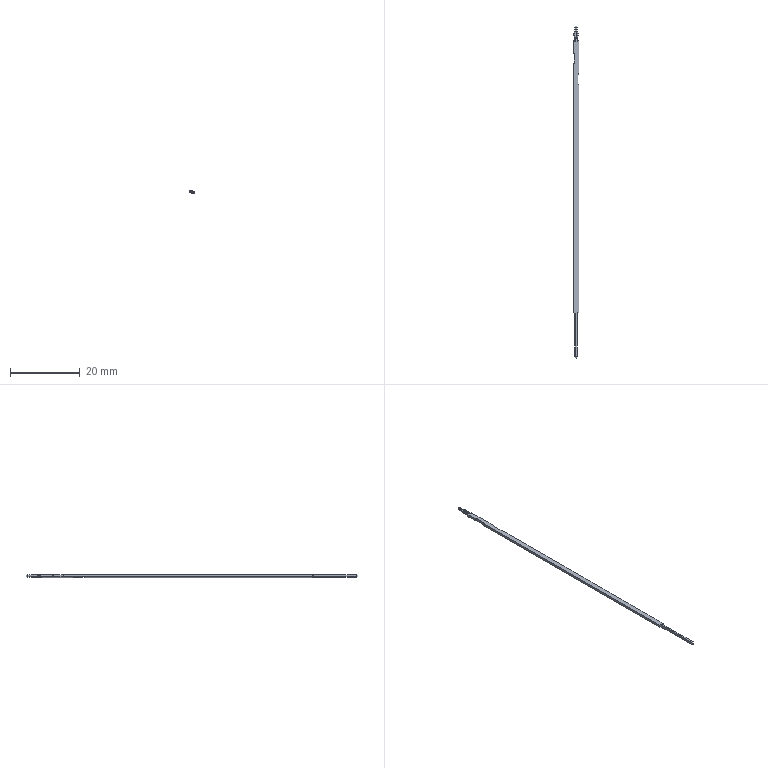Part | SolidWorks | features BaseBody 1 | 1 solid | 104 faces | box 1.687 x 95.5 x 0.9097 mm | volume 85.989 mm3 | cylinder 50 | plane 34 | torus 20 | commonest cylinder face diameters 0.2 x18 0.4 x16 8.05 x3 8.85 x3 0.165 x2 0.3 x2